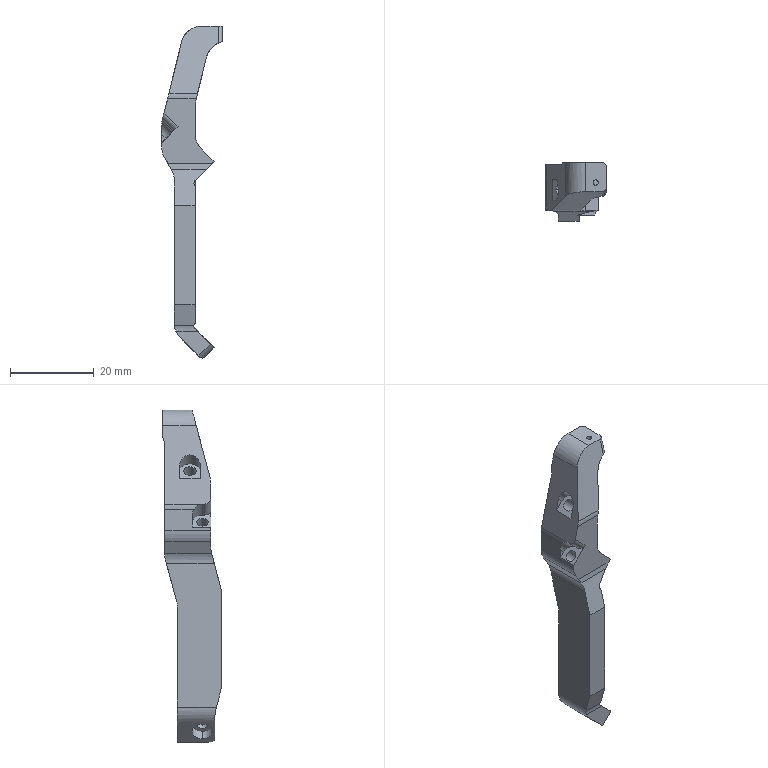Part | 1 solid | 67 faces | box 14.5 x 14 x 79.438 mm | volume 4722 mm3 | cylinder 35 | plane 32 | commonest cylinder face diameters 10 x15 2 x6 2.7 x4 5 x4 3 x3 1.25 x2